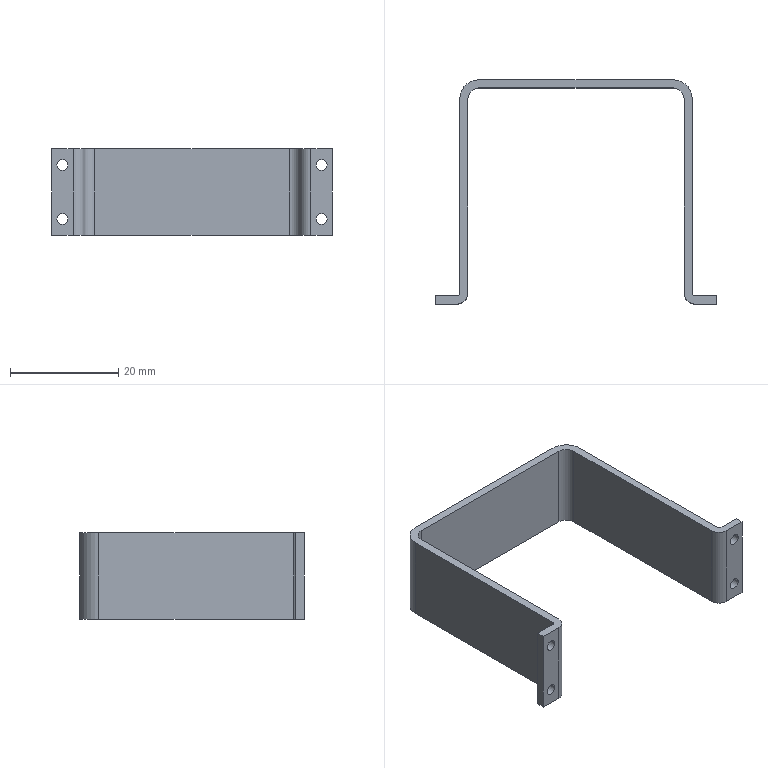Part | SolidWorks | features Extrusion 1, ICE 1 | 1 solid | 30 faces | box 52 x 41.5 x 16 mm | volume 3067 mm3 | cylinder 16 | plane 14 | commonest cylinder face diameters 2 x8 4 x4 1 x2 7 x2
STEP:
#1=CARTESIAN_POINT('',(51.,0.,13.));
#2=VERTEX_POINT('',#1);
#3=CARTESIAN_POINT('',(49.,0.,13.));
#4=VERTEX_POINT('',#3);
#5=CARTESIAN_POINT('',(50.,0.,13.));
#6=DIRECTION('',(0.,1.,0.));
#7=DIRECTION('',(-1.,0.,0.));
#8=AXIS2_PLACEMENT_3D('',#5,#6,#7);
#9=CIRCLE('',#8,1.);
#10=EDGE_CURVE('',#2,#4,#9,.T.);
#11=ORIENTED_EDGE('',*,*,#10,.F.);
#12=CARTESIAN_POINT('',(51.,1.5,13.));
#13=VERTEX_POINT('',#12);
#14=CARTESIAN_POINT('',(51.,-14.5,13.));
#15=DIRECTION('',(0.,1.,0.));
#16=VECTOR('',#15,1000.);
#17=LINE('',#14,#16);
#18=EDGE_CURVE('',#2,#13,#17,.T.);
#19=ORIENTED_EDGE('',*,*,#18,.T.);
#20=CARTESIAN_POINT('',(49.,1.5,13.));
#21=VERTEX_POINT('',#20);
#22=CARTESIAN_POINT('',(50.,1.5,13.));
#23=DIRECTION('',(0.,1.,0.));
#24=DIRECTION('',(-1.,0.,0.));
#25=AXIS2_PLACEMENT_3D('',#22,#23,#24);
#26=CIRCLE('',#25,1.);
#27=EDGE_CURVE('',#13,#21,#26,.T.);
#28=ORIENTED_EDGE('',*,*,#27,.T.);
#29=CARTESIAN_POINT('',(49.,-14.5,13.));
#30=DIRECTION('',(0.,1.,0.));
#31=VECTOR('',#30,1000.);
#32=LINE('',#29,#31);
#33=EDGE_CURVE('',#4,#21,#32,.T.);
#34=ORIENTED_EDGE('',*,*,#33,.F.);
#35=EDGE_LOOP('',(#11,#19,#28,#34));
#36=FACE_OUTER_BOUND('',#35,.T.);
#37=CARTESIAN_POINT('',(50.,-14.5,13.));
#38=DIRECTION('',(0.,1.,0.));
#39=DIRECTION('',(-1.,0.,0.));
#40=AXIS2_PLACEMENT_3D('',#37,#38,#39);
#41=CYLINDRICAL_SURFACE('',#40,1.);
#42=ADVANCED_FACE('',(#36),#41,.F.);
#43=CARTESIAN_POINT('',(3.,0.,3.));
#44=VERTEX_POINT('',#43);
#45=CARTESIAN_POINT('',(1.,0.,3.));
#46=VERTEX_POINT('',#45);
#47=CARTESIAN_POINT('',(2.,0.,3.));
#48=DIRECTION('',(0.,1.,0.));
#49=DIRECTION('',(0.,0.,1.));
#50=AXIS2_PLACEMENT_3D('',#47,#48,#49);
#51=CIRCLE('',#50,1.);
#52=EDGE_CURVE('',#44,#46,#51,.T.);
#53=ORIENTED_EDGE('',*,*,#52,.F.);
#54=CARTESIAN_POINT('',(3.,1.5,3.));
#55=VERTEX_POINT('',#54);
#56=CARTESIAN_POINT('',(3.,-14.5,3.));
#57=DIRECTION('',(0.,1.,0.));
#58=VECTOR('',#57,1000.);
#59=LINE('',#56,#58);
#60=EDGE_CURVE('',#44,#55,#59,.T.);
#61=ORIENTED_EDGE('',*,*,#60,.T.);
#62=CARTESIAN_POINT('',(1.,1.5,3.));
#63=VERTEX_POINT('',#62);
#64=CARTESIAN_POINT('',(2.,1.5,3.));
#65=DIRECTION('',(0.,1.,0.));
#66=DIRECTION('',(-1.,0.,0.));
#67=AXIS2_PLACEMENT_3D('',#64,#65,#66);
#68=CIRCLE('',#67,1.);
#69=EDGE_CURVE('',#55,#63,#68,.T.);
#70=ORIENTED_EDGE('',*,*,#69,.T.);
#71=CARTESIAN_POINT('',(1.,-14.5,3.));
#72=DIRECTION('',(0.,1.,0.));
#73=VECTOR('',#72,1000.);
#74=LINE('',#71,#73);
#75=EDGE_CURVE('',#46,#63,#74,.T.);
#76=ORIENTED_EDGE('',*,*,#75,.F.);
#77=EDGE_LOOP('',(#53,#61,#70,#76));
#78=FACE_OUTER_BOUND('',#77,.T.);
#79=CARTESIAN_POINT('',(2.,-14.5,3.));
#80=DIRECTION('',(0.,1.,0.));
#81=DIRECTION('',(-1.,0.,0.));
#82=AXIS2_PLACEMENT_3D('',#79,#80,#81);
#83=CYLINDRICAL_SURFACE('',#82,1.);
#84=ADVANCED_FACE('',(#78),#83,.F.);
#85=CARTESIAN_POINT('',(3.,0.,13.));
#86=VERTEX_POINT('',#85);
#87=CARTESIAN_POINT('',(1.,0.,13.));
#88=VERTEX_POINT('',#87);
#89=CARTESIAN_POINT('',(2.,0.,13.));
#90=DIRECTION('',(0.,1.,0.));
#91=DIRECTION('',(0.,0.,1.));
#92=AXIS2_PLACEMENT_3D('',#89,#90,#91);
#93=CIRCLE('',#92,1.);
#94=EDGE_CURVE('',#86,#88,#93,.T.);
#95=ORIENTED_EDGE('',*,*,#94,.F.);
#96=CARTESIAN_POINT('',(3.,1.5,13.));
#97=VERTEX_POINT('',#96);
#98=CARTESIAN_POINT('',(3.,-14.5,13.));
#99=DIRECTION('',(0.,1.,0.));
#100=VECTOR('',#99,1000.);
#101=LINE('',#98,#100);
#102=EDGE_CURVE('',#86,#97,#101,.T.);
#103=ORIENTED_EDGE('',*,*,#102,.T.);
#104=CARTESIAN_POINT('',(1.,1.5,13.));
#105=VERTEX_POINT('',#104);
#106=CARTESIAN_POINT('',(2.,1.5,13.));
#107=DIRECTION('',(0.,1.,0.));
#108=DIRECTION('',(-1.,0.,0.));
#109=AXIS2_PLACEMENT_3D('',#106,#107,#108);
#110=CIRCLE('',#109,1.);
#111=EDGE_CURVE('',#97,#105,#110,.T.);
#112=ORIENTED_EDGE('',*,*,#111,.T.);
#113=CARTESIAN_POINT('',(1.,-14.5,13.));
#114=DIRECTION('',(0.,1.,0.));
#115=VECTOR('',#114,1000.);
#116=LINE('',#113,#115);
#117=EDGE_CURVE('',#88,#105,#116,.T.);
#118=ORIENTED_EDGE('',*,*,#117,.F.);
#119=EDGE_LOOP('',(#95,#103,#112,#118));
#120=FACE_OUTER_BOUND('',#119,.T.);
#121=CARTESIAN_POINT('',(2.,-14.5,13.));
#122=DIRECTION('',(0.,1.,0.));
#123=DIRECTION('',(-1.,0.,0.));
#124=AXIS2_PLACEMENT_3D('',#121,#122,#123);
#125=CYLINDRICAL_SURFACE('',#124,1.);
#126=ADVANCED_FACE('',(#120),#125,.F.);
#127=CARTESIAN_POINT('',(51.,0.,3.));
#128=VERTEX_POINT('',#127);
#129=CARTESIAN_POINT('',(49.,0.,3.));
#130=VERTEX_POINT('',#129);
#131=CARTESIAN_POINT('',(50.,0.,3.));
#132=DIRECTION('',(0.,1.,0.));
#133=DIRECTION('',(-1.,0.,0.));
#134=AXIS2_PLACEMENT_3D('',#131,#132,#133);
#135=CIRCLE('',#134,1.);
#136=EDGE_CURVE('',#128,#130,#135,.T.);
#137=ORIENTED_EDGE('',*,*,#136,.F.);
#138=CARTESIAN_POINT('',(51.,1.5,3.));
#139=VERTEX_POINT('',#138);
#140=CARTESIAN_POINT('',(51.,-14.5,3.));
#141=DIRECTION('',(0.,1.,0.));
#142=VECTOR('',#141,1000.);
#143=LINE('',#140,#142);
#144=EDGE_CURVE('',#128,#139,#143,.T.);
#145=ORIENTED_EDGE('',*,*,#144,.T.);
#146=CARTESIAN_POINT('',(49.,1.5,3.));
#147=VERTEX_POINT('',#146);
#148=CARTESIAN_POINT('',(50.,1.5,3.));
#149=DIRECTION('',(0.,1.,0.));
#150=DIRECTION('',(-1.,0.,0.));
#151=AXIS2_PLACEMENT_3D('',#148,#149,#150);
#152=CIRCLE('',#151,1.);
#153=EDGE_CURVE('',#139,#147,#152,.T.);
#154=ORIENTED_EDGE('',*,*,#153,.T.);
#155=CARTESIAN_POINT('',(49.,-14.5,3.));
#156=DIRECTION('',(0.,1.,0.));
#157=VECTOR('',#156,1000.);
#158=LINE('',#155,#157);
#159=EDGE_CURVE('',#130,#147,#158,.T.);
#160=ORIENTED_EDGE('',*,*,#159,.F.);
#161=EDGE_LOOP('',(#137,#145,#154,#160));
#162=FACE_OUTER_BOUND('',#161,.T.);
#163=CARTESIAN_POINT('',(50.,-14.5,3.));
#164=DIRECTION('',(0.,1.,0.));
#165=DIRECTION('',(-1.,0.,0.));
#166=AXIS2_PLACEMENT_3D('',#163,#164,#165);
#167=CYLINDRICAL_SURFACE('',#166,1.);
#168=ADVANCED_FACE('',(#162),#167,.F.);
#169=CARTESIAN_POINT('',(0.,1.5,0.));
#170=VERTEX_POINT('',#169);
#171=CARTESIAN_POINT('',(0.,0.,0.));
#172=VERTEX_POINT('',#171);
#173=CARTESIAN_POINT('',(0.,1.5,0.));
#174=DIRECTION('',(0.,-1.,0.));
#175=VECTOR('',#174,1000.);
#176=LINE('',#173,#175);
#177=EDGE_CURVE('',#170,#172,#176,.T.);
#178=ORIENTED_EDGE('',*,*,#177,.T.);
#179=CARTESIAN_POINT('',(0.,0.,16.));
#180=VERTEX_POINT('',#179);
#181=CARTESIAN_POINT('',(0.,0.,16.));
#182=DIRECTION('',(0.,0.,-1.));
#183=VECTOR('',#182,1000.);
#184=LINE('',#181,#183);
#185=EDGE_CURVE('',#180,#172,#184,.T.);
#186=ORIENTED_EDGE('',*,*,#185,.F.);
#187=CARTESIAN_POINT('',(0.,1.5,16.));
#188=VERTEX_POINT('',#187);
#189=CARTESIAN_POINT('',(0.,1.5,16.));
#190=DIRECTION('',(0.,-1.,0.));
#191=VECTOR('',#190,1000.);
#192=LINE('',#189,#191);
#193=EDGE_CURVE('',#188,#180,#192,.T.);
#194=ORIENTED_EDGE('',*,*,#193,.F.);
#195=CARTESIAN_POINT('',(0.,1.5,16.));
#196=DIRECTION('',(0.,0.,-1.));
#197=VECTOR('',#196,1000.);
#198=LINE('',#195,#197);
#199=EDGE_CURVE('',#188,#170,#198,.T.);
#200=ORIENTED_EDGE('',*,*,#199,.T.);
#201=EDGE_LOOP('',(#178,#186,#194,#200));
#202=FACE_OUTER_BOUND('',#201,.T.);
#203=CARTESIAN_POINT('',(0.,1.5,16.));
#204=DIRECTION('',(1.,0.,0.));
#205=DIRECTION('',(0.,0.,-1.));
#206=AXIS2_PLACEMENT_3D('',#203,#204,#205);
#207=PLANE('',#206);
#208=ADVANCED_FACE('',(#202),#207,.F.);
#209=CARTESIAN_POINT('',(2.,0.,3.));
#210=DIRECTION('',(0.,1.,0.));
#211=DIRECTION('',(0.,0.,1.));
#212=AXIS2_PLACEMENT_3D('',#209,#210,#211);
#213=CIRCLE('',#212,1.);
#214=EDGE_CURVE('',#46,#44,#213,.T.);
#215=ORIENTED_EDGE('',*,*,#214,.T.);
#216=ORIENTED_EDGE('',*,*,#52,.T.);
#217=EDGE_LOOP('',(#215,#216));
#218=FACE_BOUND('',#217,.T.);
#219=CARTESIAN_POINT('',(2.,0.,13.));
#220=DIRECTION('',(0.,1.,0.));
#221=DIRECTION('',(0.,0.,1.));
#222=AXIS2_PLACEMENT_3D('',#219,#220,#221);
#223=CIRCLE('',#222,1.);
#224=EDGE_CURVE('',#88,#86,#223,.T.);
#225=ORIENTED_EDGE('',*,*,#224,.T.);
#226=ORIENTED_EDGE('',*,*,#94,.T.);
#227=EDGE_LOOP('',(#225,#226));
#228=FACE_BOUND('',#227,.T.);
#229=CARTESIAN_POINT('',(4.,0.,0.));
#230=VERTEX_POINT('',#229);
#231=CARTESIAN_POINT('',(0.,0.,0.));
#232=DIRECTION('',(1.,0.,0.));
#233=VECTOR('',#232,1000.);
#234=LINE('',#231,#233);
#235=EDGE_CURVE('',#172,#230,#234,.T.);
#236=ORIENTED_EDGE('',*,*,#235,.T.);
#237=CARTESIAN_POINT('',(4.,0.,16.));
#238=VERTEX_POINT('',#237);
#239=CARTESIAN_POINT('',(4.,0.,16.));
#240=DIRECTION('',(0.,0.,-1.));
#241=VECTOR('',#240,1000.);
#242=LINE('',#239,#241);
#243=EDGE_CURVE('',#238,#230,#242,.T.);
#244=ORIENTED_EDGE('',*,*,#243,.F.);
#245=CARTESIAN_POINT('',(0.,0.,16.));
#246=DIRECTION('',(1.,0.,0.));
#247=VECTOR('',#246,1000.);
#248=LINE('',#245,#247);
#249=EDGE_CURVE('',#180,#238,#248,.T.);
#250=ORIENTED_EDGE('',*,*,#249,.F.);
#251=ORIENTED_EDGE('',*,*,#185,.T.);
#252=EDGE_LOOP('',(#236,#244,#250,#251));
#253=FACE_OUTER_BOUND('',#252,.T.);
#254=CARTESIAN_POINT('',(0.,0.,16.));
#255=DIRECTION('',(0.,1.,0.));
#256=DIRECTION('',(0.,0.,1.));
#257=AXIS2_PLACEMENT_3D('',#254,#255,#256);
#258=PLANE('',#257);
#259=ADVANCED_FACE('',(#218,#228,#253),#258,.F.);
#260=CARTESIAN_POINT('',(6.,2.,0.));
#261=VERTEX_POINT('',#260);
#262=CARTESIAN_POINT('',(4.,2.,0.));
#263=DIRECTION('',(0.,0.,1.));
#264=DIRECTION('',(1.,0.,0.));
#265=AXIS2_PLACEMENT_3D('',#262,#263,#264);
#266=CIRCLE('',#265,2.);
#267=EDGE_CURVE('',#230,#261,#266,.T.);
#268=ORIENTED_EDGE('',*,*,#267,.T.);
#269=CARTESIAN_POINT('',(6.,2.,16.));
#270=VERTEX_POINT('',#269);
#271=CARTESIAN_POINT('',(6.,2.,16.));
#272=DIRECTION('',(0.,0.,-1.));
#273=VECTOR('',#272,1000.);
#274=LINE('',#271,#273);
#275=EDGE_CURVE('',#270,#261,#274,.T.);
#276=ORIENTED_EDGE('',*,*,#275,.F.);
#277=CARTESIAN_POINT('',(4.,2.,16.));
#278=DIRECTION('',(0.,0.,1.));
#279=DIRECTION('',(1.,0.,0.));
#280=AXIS2_PLACEMENT_3D('',#277,#278,#279);
#281=CIRCLE('',#280,2.);
#282=EDGE_CURVE('',#238,#270,#281,.T.);
#283=ORIENTED_EDGE('',*,*,#282,.F.);
#284=ORIENTED_EDGE('',*,*,#243,.T.);
#285=EDGE_LOOP('',(#268,#276,#283,#284));
#286=FACE_OUTER_BOUND('',#285,.T.);
#287=CARTESIAN_POINT('',(4.,2.,16.));
#288=DIRECTION('',(0.,0.,-1.));
#289=DIRECTION('',(-1.,0.,0.));
#290=AXIS2_PLACEMENT_3D('',#287,#288,#289);
#291=CYLINDRICAL_SURFACE('',#290,2.);
#292=ADVANCED_FACE('',(#286),#291,.T.);
#293=CARTESIAN_POINT('',(6.,38.,0.));
#294=VERTEX_POINT('',#293);
#295=CARTESIAN_POINT('',(6.,2.,0.));
#296=DIRECTION('',(0.,1.,0.));
#297=VECTOR('',#296,1000.);
#298=LINE('',#295,#297);
#299=EDGE_CURVE('',#261,#294,#298,.T.);
#300=ORIENTED_EDGE('',*,*,#299,.T.);
#301=CARTESIAN_POINT('',(6.,38.,16.));
#302=VERTEX_POINT('',#301);
#303=CARTESIAN_POINT('',(6.,38.,16.));
#304=DIRECTION('',(0.,0.,-1.));
#305=VECTOR('',#304,1000.);
#306=LINE('',#303,#305);
#307=EDGE_CURVE('',#302,#294,#306,.T.);
#308=ORIENTED_EDGE('',*,*,#307,.F.);
#309=CARTESIAN_POINT('',(6.,2.,16.));
#310=DIRECTION('',(0.,1.,0.));
#311=VECTOR('',#310,1000.);
#312=LINE('',#309,#311);
#313=EDGE_CURVE('',#270,#302,#312,.T.);
#314=ORIENTED_EDGE('',*,*,#313,.F.);
#315=ORIENTED_EDGE('',*,*,#275,.T.);
#316=EDGE_LOOP('',(#300,#308,#314,#315));
#317=FACE_OUTER_BOUND('',#316,.T.);
#318=CARTESIAN_POINT('',(6.,2.,16.));
#319=DIRECTION('',(-1.,0.,0.));
#320=DIRECTION('',(0.,0.,1.));
#321=AXIS2_PLACEMENT_3D('',#318,#319,#320);
#322=PLANE('',#321);
#323=ADVANCED_FACE('',(#317),#322,.F.);
#324=CARTESIAN_POINT('',(8.,40.,0.));
#325=VERTEX_POINT('',#324);
#326=CARTESIAN_POINT('',(8.,38.,0.));
#327=DIRECTION('',(0.,0.,-1.));
#328=DIRECTION('',(-1.,0.,0.));
#329=AXIS2_PLACEMENT_3D('',#326,#327,#328);
#330=CIRCLE('',#329,2.);
#331=EDGE_CURVE('',#294,#325,#330,.T.);
#332=ORIENTED_EDGE('',*,*,#331,.T.);
#333=CARTESIAN_POINT('',(8.,40.,16.));
#334=VERTEX_POINT('',#333);
#335=CARTESIAN_POINT('',(8.,40.,16.));
#336=DIRECTION('',(0.,0.,-1.));
#337=VECTOR('',#336,1000.);
#338=LINE('',#335,#337);
#339=EDGE_CURVE('',#334,#325,#338,.T.);
#340=ORIENTED_EDGE('',*,*,#339,.F.);
#341=CARTESIAN_POINT('',(8.,38.,16.));
#342=DIRECTION('',(0.,0.,-1.));
#343=DIRECTION('',(-1.,0.,0.));
#344=AXIS2_PLACEMENT_3D('',#341,#342,#343);
#345=CIRCLE('',#344,2.);
#346=EDGE_CURVE('',#302,#334,#345,.T.);
#347=ORIENTED_EDGE('',*,*,#346,.F.);
#348=ORIENTED_EDGE('',*,*,#307,.T.);
#349=EDGE_LOOP('',(#332,#340,#347,#348));
#350=FACE_OUTER_BOUND('',#349,.T.);
#351=CARTESIAN_POINT('',(8.,38.,16.));
#352=DIRECTION('',(0.,0.,-1.));
#353=DIRECTION('',(-1.,0.,0.));
#354=AXIS2_PLACEMENT_3D('',#351,#352,#353);
#355=CYLINDRICAL_SURFACE('',#354,2.);
#356=ADVANCED_FACE('',(#350),#355,.F.);
#357=CARTESIAN_POINT('',(44.,40.,0.));
#358=VERTEX_POINT('',#357);
#359=CARTESIAN_POINT('',(8.,40.,0.));
#360=DIRECTION('',(1.,0.,0.));
#361=VECTOR('',#360,1000.);
#362=LINE('',#359,#361);
#363=EDGE_CURVE('',#325,#358,#362,.T.);
#364=ORIENTED_EDGE('',*,*,#363,.T.);
#365=CARTESIAN_POINT('',(44.,40.,16.));
#366=VERTEX_POINT('',#365);
#367=CARTESIAN_POINT('',(44.,40.,16.));
#368=DIRECTION('',(0.,0.,-1.));
#369=VECTOR('',#368,1000.);
#370=LINE('',#367,#369);
#371=EDGE_CURVE('',#366,#358,#370,.T.);
#372=ORIENTED_EDGE('',*,*,#371,.F.);
#373=CARTESIAN_POINT('',(8.,40.,16.));
#374=DIRECTION('',(1.,0.,0.));
#375=VECTOR('',#374,1000.);
#376=LINE('',#373,#375);
#377=EDGE_CURVE('',#334,#366,#376,.T.);
#378=ORIENTED_EDGE('',*,*,#377,.F.);
#379=ORIENTED_EDGE('',*,*,#339,.T.);
#380=EDGE_LOOP('',(#364,#372,#378,#379));
#381=FACE_OUTER_BOUND('',#380,.T.);
#382=CARTESIAN_POINT('',(8.,40.,16.));
#383=DIRECTION('',(0.,1.,0.));
#384=DIRECTION('',(0.,0.,1.));
#385=AXIS2_PLACEMENT_3D('',#382,#383,#384);
#386=PLANE('',#385);
#387=ADVANCED_FACE('',(#381),#386,.F.);
#388=CARTESIAN_POINT('',(46.,38.,0.));
#389=VERTEX_POINT('',#388);
#390=CARTESIAN_POINT('',(44.,38.,0.));
#391=DIRECTION('',(0.,0.,-1.));
#392=DIRECTION('',(-1.,0.,0.));
#393=AXIS2_PLACEMENT_3D('',#390,#391,#392);
#394=CIRCLE('',#393,2.);
#395=EDGE_CURVE('',#358,#389,#394,.T.);
#396=ORIENTED_EDGE('',*,*,#395,.T.);
#397=CARTESIAN_POINT('',(46.,38.,16.));
#398=VERTEX_POINT('',#397);
#399=CARTESIAN_POINT('',(46.,38.,16.));
#400=DIRECTION('',(0.,0.,-1.));
#401=VECTOR('',#400,1000.);
#402=LINE('',#399,#401);
#403=EDGE_CURVE('',#398,#389,#402,.T.);
#404=ORIENTED_EDGE('',*,*,#403,.F.);
#405=CARTESIAN_POINT('',(44.,38.,16.));
#406=DIRECTION('',(0.,0.,-1.));
#407=DIRECTION('',(-1.,0.,0.));
#408=AXIS2_PLACEMENT_3D('',#405,#406,#407);
#409=CIRCLE('',#408,2.);
#410=EDGE_CURVE('',#366,#398,#409,.T.);
#411=ORIENTED_EDGE('',*,*,#410,.F.);
#412=ORIENTED_EDGE('',*,*,#371,.T.);
#413=EDGE_LOOP('',(#396,#404,#411,#412));
#414=FACE_OUTER_BOUND('',#413,.T.);
#415=CARTESIAN_POINT('',(44.,38.,16.));
#416=DIRECTION('',(0.,0.,-1.));
#417=DIRECTION('',(-1.,0.,0.));
#418=AXIS2_PLACEMENT_3D('',#415,#416,#417);
#419=CYLINDRICAL_SURFACE('',#418,2.);
#420=ADVANCED_FACE('',(#414),#419,.F.);
#421=CARTESIAN_POINT('',(46.,2.,0.));
#422=VERTEX_POINT('',#421);
#423=CARTESIAN_POINT('',(46.,38.,0.));
#424=DIRECTION('',(0.,-1.,0.));
#425=VECTOR('',#424,1000.);
#426=LINE('',#423,#425);
#427=EDGE_CURVE('',#389,#422,#426,.T.);
#428=ORIENTED_EDGE('',*,*,#427,.T.);
#429=CARTESIAN_POINT('',(46.,2.,16.));
#430=VERTEX_POINT('',#429);
#431=CARTESIAN_POINT('',(46.,2.,16.));
#432=DIRECTION('',(0.,0.,-1.));
#433=VECTOR('',#432,1000.);
#434=LINE('',#431,#433);
#435=EDGE_CURVE('',#430,#422,#434,.T.);
#436=ORIENTED_EDGE('',*,*,#435,.F.);
#437=CARTESIAN_POINT('',(46.,38.,16.));
#438=DIRECTION('',(0.,-1.,0.));
#439=VECTOR('',#438,1000.);
#440=LINE('',#437,#439);
#441=EDGE_CURVE('',#398,#430,#440,.T.);
#442=ORIENTED_EDGE('',*,*,#441,.F.);
#443=ORIENTED_EDGE('',*,*,#403,.T.);
#444=EDGE_LOOP('',(#428,#436,#442,#443));
#445=FACE_OUTER_BOUND('',#444,.T.);
#446=CARTESIAN_POINT('',(46.,38.,16.));
#447=DIRECTION('',(1.,0.,0.));
#448=DIRECTION('',(0.,0.,-1.));
#449=AXIS2_PLACEMENT_3D('',#446,#447,#448);
#450=PLANE('',#449);
#451=ADVANCED_FACE('',(#445),#450,.F.);
#452=CARTESIAN_POINT('',(48.,0.,0.));
#453=VERTEX_POINT('',#452);
#454=CARTESIAN_POINT('',(48.,2.,0.));
#455=DIRECTION('',(0.,0.,1.));
#456=DIRECTION('',(1.,0.,0.));
#457=AXIS2_PLACEMENT_3D('',#454,#455,#456);
#458=CIRCLE('',#457,2.);
#459=EDGE_CURVE('',#422,#453,#458,.T.);
#460=ORIENTED_EDGE('',*,*,#459,.T.);
#461=CARTESIAN_POINT('',(48.,0.,16.));
#462=VERTEX_POINT('',#461);
#463=CARTESIAN_POINT('',(48.,0.,16.));
#464=DIRECTION('',(0.,0.,-1.));
#465=VECTOR('',#464,1000.);
#466=LINE('',#463,#465);
#467=EDGE_CURVE('',#462,#453,#466,.T.);
#468=ORIENTED_EDGE('',*,*,#467,.F.);
#469=CARTESIAN_POINT('',(48.,2.,16.));
#470=DIRECTION('',(0.,0.,1.));
#471=DIRECTION('',(1.,0.,0.));
#472=AXIS2_PLACEMENT_3D('',#469,#470,#471);
#473=CIRCLE('',#472,2.);
#474=EDGE_CURVE('',#430,#462,#473,.T.);
#475=ORIENTED_EDGE('',*,*,#474,.F.);
#476=ORIENTED_EDGE('',*,*,#435,.T.);
#477=EDGE_LOOP('',(#460,#468,#475,#476));
#478=FACE_OUTER_BOUND('',#477,.T.);
#479=CARTESIAN_POINT('',(48.,2.,16.));
#480=DIRECTION('',(0.,0.,-1.));
#481=DIRECTION('',(-1.,0.,0.));
#482=AXIS2_PLACEMENT_3D('',#479,#480,#481);
#483=CYLINDRICAL_SURFACE('',#482,2.);
#484=ADVANCED_FACE('',(#478),#483,.T.);
#485=CARTESIAN_POINT('',(50.,0.,13.));
#486=DIRECTION('',(0.,1.,0.));
#487=DIRECTION('',(-1.,0.,0.));
#488=AXIS2_PLACEMENT_3D('',#485,#486,#487);
#489=CIRCLE('',#488,1.);
#490=EDGE_CURVE('',#4,#2,#489,.T.);
#491=ORIENTED_EDGE('',*,*,#490,.T.);
#492=ORIENTED_EDGE('',*,*,#10,.T.);
#493=EDGE_LOOP('',(#491,#492));
#494=FACE_BOUND('',#493,.T.);
#495=CARTESIAN_POINT('',(50.,0.,3.));
#496=DIRECTION('',(0.,1.,0.));
#497=DIRECTION('',(-1.,0.,0.));
#498=AXIS2_PLACEMENT_3D('',#495,#496,#497);
#499=CIRCLE('',#498,1.);
#500=EDGE_CURVE('',#130,#128,#499,.T.);
#501=ORIENTED_EDGE('',*,*,#500,.T.);
#502=ORIENTED_EDGE('',*,*,#136,.T.);
#503=EDGE_LOOP('',(#501,#502));
#504=FACE_BOUND('',#503,.T.);
#505=CARTESIAN_POINT('',(52.,0.,0.));
#506=VERTEX_POINT('',#505);
#507=CARTESIAN_POINT('',(48.,0.,0.));
#508=DIRECTION('',(1.,0.,0.));
#509=VECTOR('',#508,1000.);
#510=LINE('',#507,#509);
#511=EDGE_CURVE('',#453,#506,#510,.T.);
#512=ORIENTED_EDGE('',*,*,#511,.T.);
#513=CARTESIAN_POINT('',(52.,0.,16.));
#514=VERTEX_POINT('',#513);
#515=CARTESIAN_POINT('',(52.,0.,16.));
#516=DIRECTION('',(0.,0.,-1.));
#517=VECTOR('',#516,1000.);
#518=LINE('',#515,#517);
#519=EDGE_CURVE('',#514,#506,#518,.T.);
#520=ORIENTED_EDGE('',*,*,#519,.F.);
#521=CARTESIAN_POINT('',(48.,0.,16.));
#522=DIRECTION('',(1.,0.,0.));
#523=VECTOR('',#522,1000.);
#524=LINE('',#521,#523);
#525=EDGE_CURVE('',#462,#514,#524,.T.);
#526=ORIENTED_EDGE('',*,*,#525,.F.);
#527=ORIENTED_EDGE('',*,*,#467,.T.);
#528=EDGE_LOOP('',(#512,#520,#526,#527));
#529=FACE_OUTER_BOUND('',#528,.T.);
#530=CARTESIAN_POINT('',(48.,0.,16.));
#531=DIRECTION('',(0.,1.,0.));
#532=DIRECTION('',(-1.,0.,0.));
#533=AXIS2_PLACEMENT_3D('',#530,#531,#532);
#534=PLANE('',#533);
#535=ADVANCED_FACE('',(#494,#504,#529),#534,.F.);
#536=CARTESIAN_POINT('',(52.,1.5,0.));
#537=VERTEX_POINT('',#536);
#538=CARTESIAN_POINT('',(52.,1.5,0.));
#539=DIRECTION('',(0.,1.,0.));
#540=VECTOR('',#539,1000.);
#541=LINE('',#538,#540);
#542=EDGE_CURVE('',#506,#537,#541,.T.);
#543=ORIENTED_EDGE('',*,*,#542,.T.);
#544=CARTESIAN_POINT('',(52.,1.5,16.));
#545=VERTEX_POINT('',#544);
#546=CARTESIAN_POINT('',(52.,1.5,16.));
#547=DIRECTION('',(0.,0.,-1.));
#548=VECTOR('',#547,1000.);
#549=LINE('',#546,#548);
#550=EDGE_CURVE('',#545,#537,#549,.T.);
#551=ORIENTED_EDGE('',*,*,#550,.F.);
#552=CARTESIAN_POINT('',(52.,1.5,16.));
#553=DIRECTION('',(0.,1.,0.));
#554=VECTOR('',#553,1000.);
#555=LINE('',#552,#554);
#556=EDGE_CURVE('',#514,#545,#555,.T.);
#557=ORIENTED_EDGE('',*,*,#556,.F.);
#558=ORIENTED_EDGE('',*,*,#519,.T.);
#559=EDGE_LOOP('',(#543,#551,#557,#558));
#560=FACE_OUTER_BOUND('',#559,.T.);
#561=CARTESIAN_POINT('',(52.,1.5,16.));
#562=DIRECTION('',(-1.,0.,0.));
#563=DIRECTION('',(0.,0.,1.));
#564=AXIS2_PLACEMENT_3D('',#561,#562,#563);
#565=PLANE('',#564);
#566=ADVANCED_FACE('',(#560),#565,.F.);
#567=CARTESIAN_POINT('',(50.,1.5,13.));
#568=DIRECTION('',(0.,1.,0.));
#569=DIRECTION('',(-1.,0.,0.));
#570=AXIS2_PLACEMENT_3D('',#567,#568,#569);
#571=CIRCLE('',#570,1.);
#572=EDGE_CURVE('',#21,#13,#571,.T.);
#573=ORIENTED_EDGE('',*,*,#572,.F.);
#574=ORIENTED_EDGE('',*,*,#27,.F.);
#575=EDGE_LOOP('',(#573,#574));
#576=FACE_BOUND('',#575,.T.);
#577=CARTESIAN_POINT('',(50.,1.5,3.));
#578=DIRECTION('',(0.,1.,0.));
#579=DIRECTION('',(-1.,0.,0.));
#580=AXIS2_PLACEMENT_3D('',#577,#578,#579);
#581=CIRCLE('',#580,1.);
#582=EDGE_CURVE('',#147,#139,#581,.T.);
#583=ORIENTED_EDGE('',*,*,#582,.F.);
#584=ORIENTED_EDGE('',*,*,#153,.F.);
#585=EDGE_LOOP('',(#583,#584));
#586=FACE_BOUND('',#585,.T.);
#587=CARTESIAN_POINT('',(48.,1.5,0.));
#588=VERTEX_POINT('',#587);
#589=CARTESIAN_POINT('',(48.,1.5,0.));
#590=DIRECTION('',(-1.,0.,0.));
#591=VECTOR('',#590,1000.);
#592=LINE('',#589,#591);
#593=EDGE_CURVE('',#537,#588,#592,.T.);
#594=ORIENTED_EDGE('',*,*,#593,.T.);
#595=CARTESIAN_POINT('',(48.,1.5,16.));
#596=VERTEX_POINT('',#595);
#597=CARTESIAN_POINT('',(48.,1.5,16.));
#598=DIRECTION('',(0.,0.,-1.));
#599=VECTOR('',#598,1000.);
#600=LINE('',#597,#599);
#601=EDGE_CURVE('',#596,#588,#600,.T.);
#602=ORIENTED_EDGE('',*,*,#601,.F.);
#603=CARTESIAN_POINT('',(48.,1.5,16.));
#604=DIRECTION('',(-1.,0.,0.));
#605=VECTOR('',#604,1000.);
#606=LINE('',#603,#605);
#607=EDGE_CURVE('',#545,#596,#606,.T.);
#608=ORIENTED_EDGE('',*,*,#607,.F.);
#609=ORIENTED_EDGE('',*,*,#550,.T.);
#610=EDGE_LOOP('',(#594,#602,#608,#609));
#611=FACE_OUTER_BOUND('',#610,.T.);
#612=CARTESIAN_POINT('',(48.,1.5,16.));
#613=DIRECTION('',(0.,-1.,0.));
#614=DIRECTION('',(1.,0.,0.));
#615=AXIS2_PLACEMENT_3D('',#612,#613,#614);
#616=PLANE('',#615);
#617=ADVANCED_FACE('',(#576,#586,#611),#616,.F.);
#618=CARTESIAN_POINT('',(47.5,2.,0.));
#619=VERTEX_POINT('',#618);
#620=CARTESIAN_POINT('',(48.,2.,0.));
#621=DIRECTION('',(0.,0.,-1.));
#622=DIRECTION('',(1.,0.,0.));
#623=AXIS2_PLACEMENT_3D('',#620,#621,#622);
#624=CIRCLE('',#623,0.5);
#625=EDGE_CURVE('',#588,#619,#624,.T.);
#626=ORIENTED_EDGE('',*,*,#625,.T.);
#627=CARTESIAN_POINT('',(47.5,2.,16.));
#628=VERTEX_POINT('',#627);
#629=CARTESIAN_POINT('',(47.5,2.,16.));
#630=DIRECTION('',(0.,0.,-1.));
#631=VECTOR('',#630,1000.);
#632=LINE('',#629,#631);
#633=EDGE_CURVE('',#628,#619,#632,.T.);
#634=ORIENTED_EDGE('',*,*,#633,.F.);
#635=CARTESIAN_POINT('',(48.,2.,16.));
#636=DIRECTION('',(0.,0.,-1.));
#637=DIRECTION('',(1.,0.,0.));
#638=AXIS2_PLACEMENT_3D('',#635,#636,#637);
#639=CIRCLE('',#638,0.5);
#640=EDGE_CURVE('',#596,#628,#639,.T.);
#641=ORIENTED_EDGE('',*,*,#640,.F.);
#642=ORIENTED_EDGE('',*,*,#601,.T.);
#643=EDGE_LOOP('',(#626,#634,#641,#642));
#644=FACE_OUTER_BOUND('',#643,.T.);
#645=CARTESIAN_POINT('',(48.,2.,16.));
#646=DIRECTION('',(0.,0.,-1.));
#647=DIRECTION('',(-1.,0.,0.));
#648=AXIS2_PLACEMENT_3D('',#645,#646,#647);
#649=CYLINDRICAL_SURFACE('',#648,0.5);
#650=ADVANCED_FACE('',(#644),#649,.F.);
#651=CARTESIAN_POINT('',(47.5,38.,0.));
#652=VERTEX_POINT('',#651);
#653=CARTESIAN_POINT('',(47.5,38.,0.));
#654=DIRECTION('',(0.,1.,0.));
#655=VECTOR('',#654,1000.);
#656=LINE('',#653,#655);
#657=EDGE_CURVE('',#619,#652,#656,.T.);
#658=ORIENTED_EDGE('',*,*,#657,.T.);
#659=CARTESIAN_POINT('',(47.5,38.,16.));
#660=VERTEX_POINT('',#659);
#661=CARTESIAN_POINT('',(47.5,38.,16.));
#662=DIRECTION('',(0.,0.,-1.));
#663=VECTOR('',#662,1000.);
#664=LINE('',#661,#663);
#665=EDGE_CURVE('',#660,#652,#664,.T.);
#666=ORIENTED_EDGE('',*,*,#665,.F.);
#667=CARTESIAN_POINT('',(47.5,38.,16.));
#668=DIRECTION('',(0.,1.,0.));
#669=VECTOR('',#668,1000.);
#670=LINE('',#667,#669);
#671=EDGE_CURVE('',#628,#660,#670,.T.);
#672=ORIENTED_EDGE('',*,*,#671,.F.);
#673=ORIENTED_EDGE('',*,*,#633,.T.);
#674=EDGE_LOOP('',(#658,#666,#672,#673));
#675=FACE_OUTER_BOUND('',#674,.T.);
#676=CARTESIAN_POINT('',(47.5,38.,16.));
#677=DIRECTION('',(-1.,0.,0.));
#678=DIRECTION('',(0.,0.,1.));
#679=AXIS2_PLACEMENT_3D('',#676,#677,#678);
#680=PLANE('',#679);
#681=ADVANCED_FACE('',(#675),#680,.F.);
#682=CARTESIAN_POINT('',(44.,41.5,0.));
#683=VERTEX_POINT('',#682);
#684=CARTESIAN_POINT('',(44.,38.,0.));
#685=DIRECTION('',(0.,0.,1.));
#686=DIRECTION('',(-1.,0.,0.));
#687=AXIS2_PLACEMENT_3D('',#684,#685,#686);
#688=CIRCLE('',#687,3.5);
#689=EDGE_CURVE('',#652,#683,#688,.T.);
#690=ORIENTED_EDGE('',*,*,#689,.T.);
#691=CARTESIAN_POINT('',(44.,41.5,16.));
#692=VERTEX_POINT('',#691);
#693=CARTESIAN_POINT('',(44.,41.5,16.));
#694=DIRECTION('',(0.,0.,-1.));
#695=VECTOR('',#694,1000.);
#696=LINE('',#693,#695);
#697=EDGE_CURVE('',#692,#683,#696,.T.);
#698=ORIENTED_EDGE('',*,*,#697,.F.);
#699=CARTESIAN_POINT('',(44.,38.,16.));
#700=DIRECTION('',(0.,0.,1.));
#701=DIRECTION('',(-1.,0.,0.));
#702=AXIS2_PLACEMENT_3D('',#699,#700,#701);
#703=CIRCLE('',#702,3.5);
#704=EDGE_CURVE('',#660,#692,#703,.T.);
#705=ORIENTED_EDGE('',*,*,#704,.F.);
#706=ORIENTED_EDGE('',*,*,#665,.T.);
#707=EDGE_LOOP('',(#690,#698,#705,#706));
#708=FACE_OUTER_BOUND('',#707,.T.);
#709=CARTESIAN_POINT('',(44.,38.,16.));
#710=DIRECTION('',(0.,0.,-1.));
#711=DIRECTION('',(-1.,0.,0.));
#712=AXIS2_PLACEMENT_3D('',#709,#710,#711);
#713=CYLINDRICAL_SURFACE('',#712,3.5);
#714=ADVANCED_FACE('',(#708),#713,.T.);
#715=CARTESIAN_POINT('',(8.,41.5,0.));
#716=VERTEX_POINT('',#715);
#717=CARTESIAN_POINT('',(8.,41.5,0.));
#718=DIRECTION('',(-1.,0.,0.));
#719=VECTOR('',#718,1000.);
#720=LINE('',#717,#719);
#721=EDGE_CURVE('',#683,#716,#720,.T.);
#722=ORIENTED_EDGE('',*,*,#721,.T.);
#723=CARTESIAN_POINT('',(8.,41.5,16.));
#724=VERTEX_POINT('',#723);
#725=CARTESIAN_POINT('',(8.,41.5,16.));
#726=DIRECTION('',(0.,0.,-1.));
#727=VECTOR('',#726,1000.);
#728=LINE('',#725,#727);
#729=EDGE_CURVE('',#724,#716,#728,.T.);
#730=ORIENTED_EDGE('',*,*,#729,.F.);
#731=CARTESIAN_POINT('',(8.,41.5,16.));
#732=DIRECTION('',(-1.,0.,0.));
#733=VECTOR('',#732,1000.);
#734=LINE('',#731,#733);
#735=EDGE_CURVE('',#692,#724,#734,.T.);
#736=ORIENTED_EDGE('',*,*,#735,.F.);
#737=ORIENTED_EDGE('',*,*,#697,.T.);
#738=EDGE_LOOP('',(#722,#730,#736,#737));
#739=FACE_OUTER_BOUND('',#738,.T.);
#740=CARTESIAN_POINT('',(8.,41.5,16.));
#741=DIRECTION('',(0.,-1.,0.));
#742=DIRECTION('',(0.,0.,-1.));
#743=AXIS2_PLACEMENT_3D('',#740,#741,#742);
#744=PLANE('',#743);
#745=ADVANCED_FACE('',(#739),#744,.F.);
#746=CARTESIAN_POINT('',(4.5,38.,0.));
#747=VERTEX_POINT('',#746);
#748=CARTESIAN_POINT('',(8.,38.,0.));
#749=DIRECTION('',(0.,0.,1.));
#750=DIRECTION('',(-1.,0.,0.));
#751=AXIS2_PLACEMENT_3D('',#748,#749,#750);
#752=CIRCLE('',#751,3.5);
#753=EDGE_CURVE('',#716,#747,#752,.T.);
#754=ORIENTED_EDGE('',*,*,#753,.T.);
#755=CARTESIAN_POINT('',(4.5,38.,16.));
#756=VERTEX_POINT('',#755);
#757=CARTESIAN_POINT('',(4.5,38.,16.));
#758=DIRECTION('',(0.,0.,-1.));
#759=VECTOR('',#758,1000.);
#760=LINE('',#757,#759);
#761=EDGE_CURVE('',#756,#747,#760,.T.);
#762=ORIENTED_EDGE('',*,*,#761,.F.);
#763=CARTESIAN_POINT('',(8.,38.,16.));
#764=DIRECTION('',(0.,0.,1.));
#765=DIRECTION('',(-1.,0.,0.));
#766=AXIS2_PLACEMENT_3D('',#763,#764,#765);
#767=CIRCLE('',#766,3.5);
#768=EDGE_CURVE('',#724,#756,#767,.T.);
#769=ORIENTED_EDGE('',*,*,#768,.F.);
#770=ORIENTED_EDGE('',*,*,#729,.T.);
#771=EDGE_LOOP('',(#754,#762,#769,#770));
#772=FACE_OUTER_BOUND('',#771,.T.);
#773=CARTESIAN_POINT('',(8.,38.,16.));
#774=DIRECTION('',(0.,0.,-1.));
#775=DIRECTION('',(-1.,0.,0.));
#776=AXIS2_PLACEMENT_3D('',#773,#774,#775);
#777=CYLINDRICAL_SURFACE('',#776,3.5);
#778=ADVANCED_FACE('',(#772),#777,.T.);
#779=CARTESIAN_POINT('',(4.5,2.,0.));
#780=VERTEX_POINT('',#779);
#781=CARTESIAN_POINT('',(4.5,2.,0.));
#782=DIRECTION('',(0.,-1.,0.));
#783=VECTOR('',#782,1000.);
#784=LINE('',#781,#783);
#785=EDGE_CURVE('',#747,#780,#784,.T.);
#786=ORIENTED_EDGE('',*,*,#785,.T.);
#787=CARTESIAN_POINT('',(4.5,2.,16.));
#788=VERTEX_POINT('',#787);
#789=CARTESIAN_POINT('',(4.5,2.,16.));
#790=DIRECTION('',(0.,0.,-1.));
#791=VECTOR('',#790,1000.);
#792=LINE('',#789,#791);
#793=EDGE_CURVE('',#788,#780,#792,.T.);
#794=ORIENTED_EDGE('',*,*,#793,.F.);
#795=CARTESIAN_POINT('',(4.5,2.,16.));
#796=DIRECTION('',(0.,-1.,0.));
#797=VECTOR('',#796,1000.);
#798=LINE('',#795,#797);
#799=EDGE_CURVE('',#756,#788,#798,.T.);
#800=ORIENTED_EDGE('',*,*,#799,.F.);
#801=ORIENTED_EDGE('',*,*,#761,.T.);
#802=EDGE_LOOP('',(#786,#794,#800,#801));
#803=FACE_OUTER_BOUND('',#802,.T.);
#804=CARTESIAN_POINT('',(4.5,2.,16.));
#805=DIRECTION('',(1.,0.,0.));
#806=DIRECTION('',(0.,0.,-1.));
#807=AXIS2_PLACEMENT_3D('',#804,#805,#806);
#808=PLANE('',#807);
#809=ADVANCED_FACE('',(#803),#808,.F.);
#810=CARTESIAN_POINT('',(4.,1.5,0.));
#811=VERTEX_POINT('',#810);
#812=CARTESIAN_POINT('',(4.,2.,0.));
#813=DIRECTION('',(0.,0.,-1.));
#814=DIRECTION('',(1.,0.,0.));
#815=AXIS2_PLACEMENT_3D('',#812,#813,#814);
#816=CIRCLE('',#815,0.5);
#817=EDGE_CURVE('',#780,#811,#816,.T.);
#818=ORIENTED_EDGE('',*,*,#817,.T.);
#819=CARTESIAN_POINT('',(4.,1.5,16.));
#820=VERTEX_POINT('',#819);
#821=CARTESIAN_POINT('',(4.,1.5,16.));
#822=DIRECTION('',(0.,0.,-1.));
#823=VECTOR('',#822,1000.);
#824=LINE('',#821,#823);
#825=EDGE_CURVE('',#820,#811,#824,.T.);
#826=ORIENTED_EDGE('',*,*,#825,.F.);
#827=CARTESIAN_POINT('',(4.,2.,16.));
#828=DIRECTION('',(0.,0.,-1.));
#829=DIRECTION('',(1.,0.,0.));
#830=AXIS2_PLACEMENT_3D('',#827,#828,#829);
#831=CIRCLE('',#830,0.5);
#832=EDGE_CURVE('',#788,#820,#831,.T.);
#833=ORIENTED_EDGE('',*,*,#832,.F.);
#834=ORIENTED_EDGE('',*,*,#793,.T.);
#835=EDGE_LOOP('',(#818,#826,#833,#834));
#836=FACE_OUTER_BOUND('',#835,.T.);
#837=CARTESIAN_POINT('',(4.,2.,16.));
#838=DIRECTION('',(0.,0.,-1.));
#839=DIRECTION('',(-1.,0.,0.));
#840=AXIS2_PLACEMENT_3D('',#837,#838,#839);
#841=CYLINDRICAL_SURFACE('',#840,0.5);
#842=ADVANCED_FACE('',(#836),#841,.F.);
#843=CARTESIAN_POINT('',(2.,1.5,3.));
#844=DIRECTION('',(0.,1.,0.));
#845=DIRECTION('',(-1.,0.,0.));
#846=AXIS2_PLACEMENT_3D('',#843,#844,#845);
#847=CIRCLE('',#846,1.);
#848=EDGE_CURVE('',#63,#55,#847,.T.);
#849=ORIENTED_EDGE('',*,*,#848,.F.);
#850=ORIENTED_EDGE('',*,*,#69,.F.);
#851=EDGE_LOOP('',(#849,#850));
#852=FACE_BOUND('',#851,.T.);
#853=CARTESIAN_POINT('',(2.,1.5,13.));
#854=DIRECTION('',(0.,1.,0.));
#855=DIRECTION('',(-1.,0.,0.));
#856=AXIS2_PLACEMENT_3D('',#853,#854,#855);
#857=CIRCLE('',#856,1.);
#858=EDGE_CURVE('',#105,#97,#857,.T.);
#859=ORIENTED_EDGE('',*,*,#858,.F.);
#860=ORIENTED_EDGE('',*,*,#111,.F.);
#861=EDGE_LOOP('',(#859,#860));
#862=FACE_BOUND('',#861,.T.);
#863=CARTESIAN_POINT('',(0.,1.5,0.));
#864=DIRECTION('',(-1.,0.,0.));
#865=VECTOR('',#864,1000.);
#866=LINE('',#863,#865);
#867=EDGE_CURVE('',#811,#170,#866,.T.);
#868=ORIENTED_EDGE('',*,*,#867,.T.);
#869=ORIENTED_EDGE('',*,*,#199,.F.);
#870=CARTESIAN_POINT('',(0.,1.5,16.));
#871=DIRECTION('',(-1.,0.,0.));
#872=VECTOR('',#871,1000.);
#873=LINE('',#870,#872);
#874=EDGE_CURVE('',#820,#188,#873,.T.);
#875=ORIENTED_EDGE('',*,*,#874,.F.);
#876=ORIENTED_EDGE('',*,*,#825,.T.);
#877=EDGE_LOOP('',(#868,#869,#875,#876));
#878=FACE_OUTER_BOUND('',#877,.T.);
#879=CARTESIAN_POINT('',(0.,1.5,16.));
#880=DIRECTION('',(0.,-1.,0.));
#881=DIRECTION('',(0.,0.,-1.));
#882=AXIS2_PLACEMENT_3D('',#879,#880,#881);
#883=PLANE('',#882);
#884=ADVANCED_FACE('',(#852,#862,#878),#883,.F.);
#885=ORIENTED_EDGE('',*,*,#193,.T.);
#886=ORIENTED_EDGE('',*,*,#249,.T.);
#887=ORIENTED_EDGE('',*,*,#282,.T.);
#888=ORIENTED_EDGE('',*,*,#313,.T.);
#889=ORIENTED_EDGE('',*,*,#346,.T.);
#890=ORIENTED_EDGE('',*,*,#377,.T.);
#891=ORIENTED_EDGE('',*,*,#410,.T.);
#892=ORIENTED_EDGE('',*,*,#441,.T.);
#893=ORIENTED_EDGE('',*,*,#474,.T.);
#894=ORIENTED_EDGE('',*,*,#525,.T.);
#895=ORIENTED_EDGE('',*,*,#556,.T.);
#896=ORIENTED_EDGE('',*,*,#607,.T.);
#897=ORIENTED_EDGE('',*,*,#640,.T.);
#898=ORIENTED_EDGE('',*,*,#671,.T.);
#899=ORIENTED_EDGE('',*,*,#704,.T.);
#900=ORIENTED_EDGE('',*,*,#735,.T.);
#901=ORIENTED_EDGE('',*,*,#768,.T.);
#902=ORIENTED_EDGE('',*,*,#799,.T.);
#903=ORIENTED_EDGE('',*,*,#832,.T.);
#904=ORIENTED_EDGE('',*,*,#874,.T.);
#905=EDGE_LOOP('',(#885,#886,#887,#888,#889,#890,#891,#892,#893,#894,#895,#896,#897,#898,#899,#900,#901,#902,#903,#904));
#906=FACE_OUTER_BOUND('',#905,.T.);
#907=CARTESIAN_POINT('',(4.,2.,16.));
#908=DIRECTION('',(0.,0.,1.));
#909=DIRECTION('',(1.,0.,0.));
#910=AXIS2_PLACEMENT_3D('',#907,#908,#909);
#911=PLANE('',#910);
#912=ADVANCED_FACE('',(#906),#911,.T.);
#913=ORIENTED_EDGE('',*,*,#177,.F.);
#914=ORIENTED_EDGE('',*,*,#867,.F.);
#915=ORIENTED_EDGE('',*,*,#817,.F.);
#916=ORIENTED_EDGE('',*,*,#785,.F.);
#917=ORIENTED_EDGE('',*,*,#753,.F.);
#918=ORIENTED_EDGE('',*,*,#721,.F.);
#919=ORIENTED_EDGE('',*,*,#689,.F.);
#920=ORIENTED_EDGE('',*,*,#657,.F.);
#921=ORIENTED_EDGE('',*,*,#625,.F.);
#922=ORIENTED_EDGE('',*,*,#593,.F.);
#923=ORIENTED_EDGE('',*,*,#542,.F.);
#924=ORIENTED_EDGE('',*,*,#511,.F.);
#925=ORIENTED_EDGE('',*,*,#459,.F.);
#926=ORIENTED_EDGE('',*,*,#427,.F.);
#927=ORIENTED_EDGE('',*,*,#395,.F.);
#928=ORIENTED_EDGE('',*,*,#363,.F.);
#929=ORIENTED_EDGE('',*,*,#331,.F.);
#930=ORIENTED_EDGE('',*,*,#299,.F.);
#931=ORIENTED_EDGE('',*,*,#267,.F.);
#932=ORIENTED_EDGE('',*,*,#235,.F.);
#933=EDGE_LOOP('',(#913,#914,#915,#916,#917,#918,#919,#920,#921,#922,#923,#924,#925,#926,#927,#928,#929,#930,#931,#932));
#934=FACE_OUTER_BOUND('',#933,.T.);
#935=CARTESIAN_POINT('',(4.,2.,0.));
#936=DIRECTION('',(0.,0.,1.));
#937=DIRECTION('',(1.,0.,0.));
#938=AXIS2_PLACEMENT_3D('',#935,#936,#937);
#939=PLANE('',#938);
#940=ADVANCED_FACE('',(#934),#939,.F.);
#941=ORIENTED_EDGE('',*,*,#144,.F.);
#942=ORIENTED_EDGE('',*,*,#500,.F.);
#943=ORIENTED_EDGE('',*,*,#159,.T.);
#944=ORIENTED_EDGE('',*,*,#582,.T.);
#945=EDGE_LOOP('',(#941,#942,#943,#944));
#946=FACE_OUTER_BOUND('',#945,.T.);
#947=CARTESIAN_POINT('',(50.,-14.5,3.));
#948=DIRECTION('',(0.,1.,0.));
#949=DIRECTION('',(-1.,0.,0.));
#950=AXIS2_PLACEMENT_3D('',#947,#948,#949);
#951=CYLINDRICAL_SURFACE('',#950,1.);
#952=ADVANCED_FACE('',(#946),#951,.F.);
#953=ORIENTED_EDGE('',*,*,#102,.F.);
#954=ORIENTED_EDGE('',*,*,#224,.F.);
#955=ORIENTED_EDGE('',*,*,#117,.T.);
#956=ORIENTED_EDGE('',*,*,#858,.T.);
#957=EDGE_LOOP('',(#953,#954,#955,#956));
#958=FACE_OUTER_BOUND('',#957,.T.);
#959=CARTESIAN_POINT('',(2.,-14.5,13.));
#960=DIRECTION('',(0.,1.,0.));
#961=DIRECTION('',(-1.,0.,0.));
#962=AXIS2_PLACEMENT_3D('',#959,#960,#961);
#963=CYLINDRICAL_SURFACE('',#962,1.);
#964=ADVANCED_FACE('',(#958),#963,.F.);
#965=ORIENTED_EDGE('',*,*,#60,.F.);
#966=ORIENTED_EDGE('',*,*,#214,.F.);
#967=ORIENTED_EDGE('',*,*,#75,.T.);
#968=ORIENTED_EDGE('',*,*,#848,.T.);
#969=EDGE_LOOP('',(#965,#966,#967,#968));
#970=FACE_OUTER_BOUND('',#969,.T.);
#971=CARTESIAN_POINT('',(2.,-14.5,3.));
#972=DIRECTION('',(0.,1.,0.));
#973=DIRECTION('',(-1.,0.,0.));
#974=AXIS2_PLACEMENT_3D('',#971,#972,#973);
#975=CYLINDRICAL_SURFACE('',#974,1.);
#976=ADVANCED_FACE('',(#970),#975,.F.);
#977=ORIENTED_EDGE('',*,*,#18,.F.);
#978=ORIENTED_EDGE('',*,*,#490,.F.);
#979=ORIENTED_EDGE('',*,*,#33,.T.);
#980=ORIENTED_EDGE('',*,*,#572,.T.);
#981=EDGE_LOOP('',(#977,#978,#979,#980));
#982=FACE_OUTER_BOUND('',#981,.T.);
#983=CARTESIAN_POINT('',(50.,-14.5,13.));
#984=DIRECTION('',(0.,1.,0.));
#985=DIRECTION('',(-1.,0.,0.));
#986=AXIS2_PLACEMENT_3D('',#983,#984,#985);
#987=CYLINDRICAL_SURFACE('',#986,1.);
#988=ADVANCED_FACE('',(#982),#987,.F.);
#989=CLOSED_SHELL('',(#42,#84,#126,#168,#208,#259,#292,#323,#356,#387,#420,#451,#484,#535,#566,#617,#650,#681,#714,#745,#778,#809,#842,#884,#912,#940,#952,#964,#976,#988));
#990=MANIFOLD_SOLID_BREP('',#989);
#991=CARTESIAN_POINT('',(0.,0.,0.));
#992=DIRECTION('',(0.,0.,1.));
#993=DIRECTION('',(1.,0.,0.));
#994=AXIS2_PLACEMENT_3D('',#991,#992,#993);
#995=(LENGTH_UNIT()NAMED_UNIT(*)SI_UNIT(.MILLI.,.METRE.));
#996=UNCERTAINTY_MEASURE_WITH_UNIT(LENGTH_MEASURE(0.00001),#995,'','');
#997=(NAMED_UNIT(*)PLANE_ANGLE_UNIT()SI_UNIT($,.RADIAN.));
#998=(NAMED_UNIT(*)SI_UNIT($,.STERADIAN.)SOLID_ANGLE_UNIT());
#999=(GEOMETRIC_REPRESENTATION_CONTEXT(3)GLOBAL_UNCERTAINTY_ASSIGNED_CONTEXT((#996))GLOBAL_UNIT_ASSIGNED_CONTEXT((#995,#997,#998))REPRESENTATION_CONTEXT('',''));
#1000=ADVANCED_BREP_SHAPE_REPRESENTATION('',(#990,#994),#999);